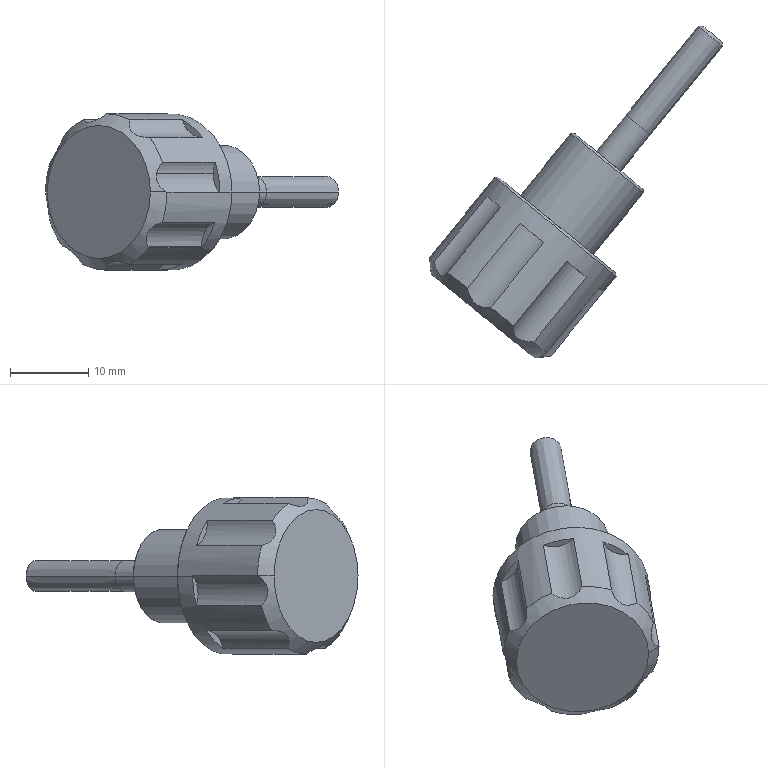Part | SolidWorks | features BaseBody 1 | 1 solid | 38 faces | box 37.447 x 42.447 x 20 mm | volume 5886 mm3 | cylinder 16 | plane 12 | cone 10 | commonest cylinder face diameters 6.478 x10 4 x2 12 x2 20 x2
STEP:
#1=CARTESIAN_POINT('',(523.226,-172.155,255.843));
#2=VERTEX_POINT('',#1);
#3=CARTESIAN_POINT('',(507.709,-159.537,255.843));
#4=VERTEX_POINT('',#3);
#5=CARTESIAN_POINT('',(515.467,-165.846,255.843));
#6=DIRECTION('',(-0.6309,-0.7758,0.000000012));
#7=DIRECTION('',(0.7758,-0.6309,0.));
#8=AXIS2_PLACEMENT_3D('',#5,#6,#7);
#9=CIRCLE('',#8,10.);
#10=EDGE_CURVE('',#2,#4,#9,.T.);
#11=ORIENTED_EDGE('',*,*,#10,.T.);
#12=CARTESIAN_POINT('',(506.127,-161.482,255.843));
#13=VERTEX_POINT('',#12);
#14=CARTESIAN_POINT('',(498.434,-170.941,255.843));
#15=DIRECTION('',(-0.6309,-0.7758,0.000000012));
#16=VECTOR('',#15,1000.);
#17=LINE('',#14,#16);
#18=EDGE_CURVE('',#4,#13,#17,.T.);
#19=ORIENTED_EDGE('',*,*,#18,.T.);
#20=CARTESIAN_POINT('',(506.127,-161.482,255.944));
#21=VERTEX_POINT('',#20);
#22=CARTESIAN_POINT('',(513.885,-167.791,255.843));
#23=DIRECTION('',(0.6309,0.7758,-0.000000012));
#24=DIRECTION('',(0.7758,-0.6309,0.));
#25=AXIS2_PLACEMENT_3D('',#22,#23,#24);
#26=CIRCLE('',#25,10.);
#27=EDGE_CURVE('',#13,#21,#26,.T.);
#28=ORIENTED_EDGE('',*,*,#27,.T.);
#29=CARTESIAN_POINT('',(499.381,-169.778,255.944));
#30=VERTEX_POINT('',#29);
#31=CARTESIAN_POINT('',(498.434,-170.942,255.944));
#32=DIRECTION('',(-0.6309,-0.7758,0.000000012));
#33=VECTOR('',#32,1000.);
#34=LINE('',#31,#33);
#35=EDGE_CURVE('',#21,#30,#34,.T.);
#36=ORIENTED_EDGE('',*,*,#35,.T.);
#37=CARTESIAN_POINT('',(499.988,-170.272,259.722));
#38=VERTEX_POINT('',#37);
#39=CARTESIAN_POINT('',(507.139,-176.087,255.843));
#40=DIRECTION('',(0.6309,0.7758,-0.000000012));
#41=DIRECTION('',(0.7758,-0.6309,0.));
#42=AXIS2_PLACEMENT_3D('',#39,#40,#41);
#43=CIRCLE('',#42,10.);
#44=EDGE_CURVE('',#30,#38,#43,.T.);
#45=ORIENTED_EDGE('',*,*,#44,.T.);
#46=CARTESIAN_POINT('',(506.734,-161.976,259.722));
#47=VERTEX_POINT('',#46);
#48=CARTESIAN_POINT('',(499.041,-171.435,259.722));
#49=DIRECTION('',(0.6309,0.7758,-0.000000012));
#50=VECTOR('',#49,1000.);
#51=LINE('',#48,#50);
#52=EDGE_CURVE('',#38,#47,#51,.T.);
#53=ORIENTED_EDGE('',*,*,#52,.T.);
#54=CARTESIAN_POINT('',(508.454,-163.375,262.985));
#55=VERTEX_POINT('',#54);
#56=CARTESIAN_POINT('',(513.885,-167.791,255.843));
#57=DIRECTION('',(0.6309,0.7758,-0.000000012));
#58=DIRECTION('',(0.7758,-0.6309,0.));
#59=AXIS2_PLACEMENT_3D('',#56,#57,#58);
#60=CIRCLE('',#59,10.);
#61=EDGE_CURVE('',#47,#55,#60,.T.);
#62=ORIENTED_EDGE('',*,*,#61,.T.);
#63=CARTESIAN_POINT('',(501.708,-171.671,262.985));
#64=VERTEX_POINT('',#63);
#65=CARTESIAN_POINT('',(500.762,-172.834,262.985));
#66=DIRECTION('',(-0.6309,-0.7758,0.000000012));
#67=VECTOR('',#66,1000.);
#68=LINE('',#65,#67);
#69=EDGE_CURVE('',#55,#64,#68,.T.);
#70=ORIENTED_EDGE('',*,*,#69,.T.);
#71=CARTESIAN_POINT('',(504.21,-173.705,265.104));
#72=VERTEX_POINT('',#71);
#73=CARTESIAN_POINT('',(507.139,-176.087,255.843));
#74=DIRECTION('',(0.6309,0.7758,-0.000000012));
#75=DIRECTION('',(0.7758,-0.6309,0.));
#76=AXIS2_PLACEMENT_3D('',#73,#74,#75);
#77=CIRCLE('',#76,10.);
#78=EDGE_CURVE('',#64,#72,#77,.T.);
#79=ORIENTED_EDGE('',*,*,#78,.T.);
#80=CARTESIAN_POINT('',(510.956,-165.41,265.104));
#81=VERTEX_POINT('',#80);
#82=CARTESIAN_POINT('',(503.264,-174.869,265.104));
#83=DIRECTION('',(0.6309,0.7758,-0.000000012));
#84=VECTOR('',#83,1000.);
#85=LINE('',#82,#84);
#86=EDGE_CURVE('',#72,#81,#85,.T.);
#87=ORIENTED_EDGE('',*,*,#86,.T.);
#88=CARTESIAN_POINT('',(513.963,-167.855,265.843));
#89=VERTEX_POINT('',#88);
#90=CARTESIAN_POINT('',(513.885,-167.791,255.843));
#91=DIRECTION('',(0.6309,0.7758,-0.000000012));
#92=DIRECTION('',(0.7758,-0.6309,0.));
#93=AXIS2_PLACEMENT_3D('',#90,#91,#92);
#94=CIRCLE('',#93,10.);
#95=EDGE_CURVE('',#81,#89,#94,.T.);
#96=ORIENTED_EDGE('',*,*,#95,.T.);
#97=CARTESIAN_POINT('',(507.217,-176.15,265.843));
#98=VERTEX_POINT('',#97);
#99=CARTESIAN_POINT('',(506.271,-177.314,265.843));
#100=DIRECTION('',(-0.6309,-0.7758,0.000000012));
#101=VECTOR('',#100,1000.);
#102=LINE('',#99,#101);
#103=EDGE_CURVE('',#89,#98,#102,.T.);
#104=ORIENTED_EDGE('',*,*,#103,.T.);
#105=CARTESIAN_POINT('',(510.148,-178.534,265.06));
#106=VERTEX_POINT('',#105);
#107=CARTESIAN_POINT('',(507.139,-176.087,255.843));
#108=DIRECTION('',(0.6309,0.7758,-0.000000012));
#109=DIRECTION('',(0.7758,-0.6309,0.));
#110=AXIS2_PLACEMENT_3D('',#107,#108,#109);
#111=CIRCLE('',#110,10.);
#112=EDGE_CURVE('',#98,#106,#111,.T.);
#113=ORIENTED_EDGE('',*,*,#112,.T.);
#114=CARTESIAN_POINT('',(516.894,-170.239,265.06));
#115=VERTEX_POINT('',#114);
#116=CARTESIAN_POINT('',(509.202,-179.698,265.06));
#117=DIRECTION('',(0.6309,0.7758,-0.000000012));
#118=VECTOR('',#117,1000.);
#119=LINE('',#116,#118);
#120=EDGE_CURVE('',#106,#115,#119,.T.);
#121=ORIENTED_EDGE('',*,*,#120,.T.);
#122=CARTESIAN_POINT('',(519.426,-172.297,262.843));
#123=VERTEX_POINT('',#122);
#124=CARTESIAN_POINT('',(513.885,-167.791,255.843));
#125=DIRECTION('',(0.6309,0.7758,-0.000000012));
#126=DIRECTION('',(0.7758,-0.6309,0.));
#127=AXIS2_PLACEMENT_3D('',#124,#125,#126);
#128=CIRCLE('',#127,10.);
#129=EDGE_CURVE('',#115,#123,#128,.T.);
#130=ORIENTED_EDGE('',*,*,#129,.T.);
#131=CARTESIAN_POINT('',(512.68,-180.593,262.843));
#132=VERTEX_POINT('',#131);
#133=CARTESIAN_POINT('',(511.733,-181.757,262.843));
#134=DIRECTION('',(-0.6309,-0.7758,0.000000012));
#135=VECTOR('',#134,1000.);
#136=LINE('',#133,#135);
#137=EDGE_CURVE('',#123,#132,#136,.T.);
#138=ORIENTED_EDGE('',*,*,#137,.T.);
#139=CARTESIAN_POINT('',(514.323,-181.929,259.618));
#140=VERTEX_POINT('',#139);
#141=CARTESIAN_POINT('',(507.139,-176.087,255.843));
#142=DIRECTION('',(0.6309,0.7758,-0.000000012));
#143=DIRECTION('',(0.7758,-0.6309,0.));
#144=AXIS2_PLACEMENT_3D('',#141,#142,#143);
#145=CIRCLE('',#144,10.);
#146=EDGE_CURVE('',#132,#140,#145,.T.);
#147=ORIENTED_EDGE('',*,*,#146,.T.);
#148=CARTESIAN_POINT('',(521.069,-173.634,259.618));
#149=VERTEX_POINT('',#148);
#150=CARTESIAN_POINT('',(513.377,-183.093,259.618));
#151=DIRECTION('',(0.6309,0.7758,-0.000000012));
#152=VECTOR('',#151,1000.);
#153=LINE('',#150,#152);
#154=EDGE_CURVE('',#140,#149,#153,.T.);
#155=ORIENTED_EDGE('',*,*,#154,.T.);
#156=CARTESIAN_POINT('',(521.643,-174.101,255.843));
#157=VERTEX_POINT('',#156);
#158=CARTESIAN_POINT('',(513.885,-167.791,255.843));
#159=DIRECTION('',(0.6309,0.7758,-0.000000012));
#160=DIRECTION('',(0.7758,-0.6309,0.));
#161=AXIS2_PLACEMENT_3D('',#158,#159,#160);
#162=CIRCLE('',#161,10.);
#163=EDGE_CURVE('',#149,#157,#162,.T.);
#164=ORIENTED_EDGE('',*,*,#163,.T.);
#165=CARTESIAN_POINT('',(513.951,-183.56,255.843));
#166=DIRECTION('',(-0.6309,-0.7758,0.000000012));
#167=VECTOR('',#166,1000.);
#168=LINE('',#165,#167);
#169=EDGE_CURVE('',#2,#157,#168,.T.);
#170=ORIENTED_EDGE('',*,*,#169,.F.);
#171=EDGE_LOOP('',(#11,#19,#28,#36,#45,#53,#62,#70,#79,#87,#96,#104,#113,#121,#130,#138,#147,#155,#164,#170));
#172=FACE_OUTER_BOUND('',#171,.T.);
#173=CARTESIAN_POINT('',(506.192,-177.251,255.843));
#174=DIRECTION('',(-0.6309,-0.7758,0.000000012));
#175=DIRECTION('',(0.7758,-0.6309,0.));
#176=AXIS2_PLACEMENT_3D('',#173,#174,#175);
#177=CYLINDRICAL_SURFACE('',#176,10.);
#178=ADVANCED_FACE('',(#172),#177,.T.);
#179=CARTESIAN_POINT('',(499.598,-171.888,255.843));
#180=VERTEX_POINT('',#179);
#181=CARTESIAN_POINT('',(512.787,-182.614,255.843));
#182=VERTEX_POINT('',#181);
#183=CARTESIAN_POINT('',(506.192,-177.251,255.843));
#184=DIRECTION('',(0.6309,0.7758,-0.000000012));
#185=DIRECTION('',(-0.7758,0.6309,0.));
#186=AXIS2_PLACEMENT_3D('',#183,#184,#185);
#187=CIRCLE('',#186,8.5);
#188=EDGE_CURVE('',#180,#182,#187,.T.);
#189=ORIENTED_EDGE('',*,*,#188,.T.);
#190=CARTESIAN_POINT('',(514.745,-182.412,255.843));
#191=VERTEX_POINT('',#190);
#192=CARTESIAN_POINT('',(514.897,-182.396,255.843));
#193=DIRECTION('',(0.9947,0.1025,-0.000000009));
#194=VECTOR('',#193,1000.);
#195=LINE('',#192,#194);
#196=EDGE_CURVE('',#182,#191,#195,.T.);
#197=ORIENTED_EDGE('',*,*,#196,.T.);
#198=CARTESIAN_POINT('',(513.557,-182.323,258.162));
#199=VERTEX_POINT('',#198);
#200=CARTESIAN_POINT('',(514.745,-182.412,255.843));
#201=CARTESIAN_POINT('',(514.556,-182.431,255.974));
#202=CARTESIAN_POINT('',(514.379,-182.448,256.12));
#203=CARTESIAN_POINT('',(514.058,-182.47,256.452));
#204=CARTESIAN_POINT('',(513.915,-182.475,256.636));
#205=CARTESIAN_POINT('',(513.746,-182.469,256.937));
#206=CARTESIAN_POINT('',(513.697,-182.464,257.043));
#207=CARTESIAN_POINT('',(513.617,-182.45,257.259));
#208=CARTESIAN_POINT('',(513.586,-182.441,257.369));
#209=CARTESIAN_POINT('',(513.523,-182.404,257.704));
#210=CARTESIAN_POINT('',(513.522,-182.367,257.938));
#211=CARTESIAN_POINT('',(513.557,-182.323,258.162));
#212=B_SPLINE_CURVE_WITH_KNOTS('',3,(#200,#201,#202,#203,#204,#205,#206,#207,#208,#209,#210,#211),.UNSPECIFIED.,.F.,.F.,(4,2,2,2,2,4),(0.0001822,0.0008713,0.00156,0.001905,0.00225,0.002939),.UNSPECIFIED.);
#213=EDGE_CURVE('',#191,#199,#212,.T.);
#214=ORIENTED_EDGE('',*,*,#213,.T.);
#215=CARTESIAN_POINT('',(513.557,-182.323,258.162));
#216=CARTESIAN_POINT('',(513.579,-182.296,258.3));
#217=CARTESIAN_POINT('',(513.615,-182.266,258.437));
#218=CARTESIAN_POINT('',(513.709,-182.203,258.7));
#219=CARTESIAN_POINT('',(513.767,-182.17,258.825));
#220=CARTESIAN_POINT('',(513.966,-182.069,259.188));
#221=CARTESIAN_POINT('',(514.134,-181.999,259.413));
#222=CARTESIAN_POINT('',(514.323,-181.929,259.618));
#223=B_SPLINE_CURVE_WITH_KNOTS('',3,(#215,#216,#217,#218,#219,#220,#221,#222),.UNSPECIFIED.,.F.,.F.,(4,2,2,4),(0.002939,0.003365,0.003792,0.004644),.UNSPECIFIED.);
#224=EDGE_CURVE('',#199,#140,#223,.T.);
#225=ORIENTED_EDGE('',*,*,#224,.T.);
#226=ORIENTED_EDGE('',*,*,#146,.F.);
#227=CARTESIAN_POINT('',(512.68,-180.593,262.843));
#228=CARTESIAN_POINT('',(512.485,-180.586,262.834));
#229=CARTESIAN_POINT('',(512.292,-180.571,262.836));
#230=CARTESIAN_POINT('',(511.909,-180.523,262.865));
#231=CARTESIAN_POINT('',(511.717,-180.489,262.893));
#232=CARTESIAN_POINT('',(511.35,-180.396,262.981));
#233=CARTESIAN_POINT('',(511.175,-180.337,263.039));
#234=CARTESIAN_POINT('',(510.847,-180.189,263.194));
#235=CARTESIAN_POINT('',(510.7,-180.1,263.288));
#236=CARTESIAN_POINT('',(510.448,-179.895,263.509));
#237=CARTESIAN_POINT('',(510.349,-179.783,263.63));
#238=CARTESIAN_POINT('',(510.197,-179.544,263.893));
#239=CARTESIAN_POINT('',(510.145,-179.417,264.035));
#240=CARTESIAN_POINT('',(510.085,-179.163,264.322));
#241=CARTESIAN_POINT('',(510.075,-179.034,264.469));
#242=CARTESIAN_POINT('',(510.089,-178.781,264.764));
#243=CARTESIAN_POINT('',(510.112,-178.656,264.912));
#244=CARTESIAN_POINT('',(510.148,-178.534,265.06));
#245=B_SPLINE_CURVE_WITH_KNOTS('',3,(#227,#228,#229,#230,#231,#232,#233,#234,#235,#236,#237,#238,#239,#240,#241,#242,#243,#244),.UNSPECIFIED.,.F.,.F.,(4,2,2,2,2,2,2,2,4),(0.,0.0005805,0.001161,0.001742,0.002322,0.002903,0.003483,0.004064,0.004644),.UNSPECIFIED.);
#246=EDGE_CURVE('',#132,#106,#245,.T.);
#247=ORIENTED_EDGE('',*,*,#246,.T.);
#248=ORIENTED_EDGE('',*,*,#112,.F.);
#249=CARTESIAN_POINT('',(507.217,-176.15,265.843));
#250=CARTESIAN_POINT('',(507.062,-176.176,265.726));
#251=CARTESIAN_POINT('',(506.904,-176.19,265.615));
#252=CARTESIAN_POINT('',(506.579,-176.189,265.404));
#253=CARTESIAN_POINT('',(506.411,-176.174,265.304));
#254=CARTESIAN_POINT('',(506.074,-176.106,265.123));
#255=CARTESIAN_POINT('',(505.906,-176.053,265.042));
#256=CARTESIAN_POINT('',(505.573,-175.899,264.905));
#257=CARTESIAN_POINT('',(505.414,-175.801,264.852));
#258=CARTESIAN_POINT('',(505.119,-175.562,264.779));
#259=CARTESIAN_POINT('',(504.982,-175.419,264.76));
#260=CARTESIAN_POINT('',(504.746,-175.111,264.756));
#261=CARTESIAN_POINT('',(504.643,-174.942,264.771));
#262=CARTESIAN_POINT('',(504.387,-174.427,264.855));
#263=CARTESIAN_POINT('',(504.278,-174.064,264.963));
#264=CARTESIAN_POINT('',(504.21,-173.705,265.104));
#265=B_SPLINE_CURVE_WITH_KNOTS('',3,(#249,#250,#251,#252,#253,#254,#255,#256,#257,#258,#259,#260,#261,#262,#263,#264),.UNSPECIFIED.,.F.,.F.,(4,2,2,2,2,2,2,4),(0.,0.0005805,0.001161,0.001742,0.002322,0.002903,0.003483,0.004644),.UNSPECIFIED.);
#266=EDGE_CURVE('',#98,#72,#265,.T.);
#267=ORIENTED_EDGE('',*,*,#266,.T.);
#268=ORIENTED_EDGE('',*,*,#78,.F.);
#269=CARTESIAN_POINT('',(501.708,-171.671,262.985));
#270=CARTESIAN_POINT('',(501.641,-171.768,262.83));
#271=CARTESIAN_POINT('',(501.57,-171.852,262.67));
#272=CARTESIAN_POINT('',(501.418,-171.992,262.343));
#273=CARTESIAN_POINT('',(501.337,-172.048,262.173));
#274=CARTESIAN_POINT('',(501.168,-172.116,261.829));
#275=CARTESIAN_POINT('',(501.082,-172.13,261.656));
#276=CARTESIAN_POINT('',(500.905,-172.103,261.308));
#277=CARTESIAN_POINT('',(500.817,-172.062,261.14));
#278=CARTESIAN_POINT('',(500.648,-171.926,260.82));
#279=CARTESIAN_POINT('',(500.566,-171.828,260.667));
#280=CARTESIAN_POINT('',(500.418,-171.592,260.397));
#281=CARTESIAN_POINT('',(500.35,-171.451,260.276));
#282=CARTESIAN_POINT('',(500.167,-170.995,259.966));
#283=CARTESIAN_POINT('',(500.069,-170.641,259.82));
#284=CARTESIAN_POINT('',(499.988,-170.272,259.722));
#285=B_SPLINE_CURVE_WITH_KNOTS('',3,(#269,#270,#271,#272,#273,#274,#275,#276,#277,#278,#279,#280,#281,#282,#283,#284),.UNSPECIFIED.,.F.,.F.,(4,2,2,2,2,2,2,4),(0.,0.0005805,0.001161,0.001742,0.002322,0.002903,0.003483,0.004644),.UNSPECIFIED.);
#286=EDGE_CURVE('',#64,#38,#285,.T.);
#287=ORIENTED_EDGE('',*,*,#286,.T.);
#288=ORIENTED_EDGE('',*,*,#44,.F.);
#289=CARTESIAN_POINT('',(499.396,-169.93,255.843));
#290=VERTEX_POINT('',#289);
#291=CARTESIAN_POINT('',(499.381,-169.778,255.944));
#292=CARTESIAN_POINT('',(499.386,-169.83,255.911));
#293=CARTESIAN_POINT('',(499.391,-169.88,255.878));
#294=CARTESIAN_POINT('',(499.396,-169.93,255.843));
#295=B_SPLINE_CURVE_WITH_KNOTS('',3,(#291,#292,#293,#294),.UNSPECIFIED.,.F.,.F.,(4,4),(0.,0.0001822),.UNSPECIFIED.);
#296=EDGE_CURVE('',#30,#290,#295,.T.);
#297=ORIENTED_EDGE('',*,*,#296,.T.);
#298=CARTESIAN_POINT('',(499.38,-169.778,255.843));
#299=DIRECTION('',(-0.1025,0.9947,-0.000000009));
#300=VECTOR('',#299,1000.);
#301=LINE('',#298,#300);
#302=EDGE_CURVE('',#180,#290,#301,.T.);
#303=ORIENTED_EDGE('',*,*,#302,.F.);
#304=EDGE_LOOP('',(#189,#197,#214,#225,#226,#247,#248,#267,#268,#287,#288,#297,#303));
#305=FACE_OUTER_BOUND('',#304,.T.);
#306=CARTESIAN_POINT('',(507.139,-176.087,255.843));
#307=DIRECTION('',(0.6309,0.7758,-0.000000012));
#308=DIRECTION('',(-0.7758,0.6309,0.));
#309=AXIS2_PLACEMENT_3D('',#306,#307,#308);
#310=CONICAL_SURFACE('',#309,10.,0.7854);
#311=ADVANCED_FACE('',(#305),#310,.T.);
#312=CARTESIAN_POINT('',(512.479,-180.606,248.889));
#313=VERTEX_POINT('',#312);
#314=CARTESIAN_POINT('',(514.29,-181.902,251.964));
#315=VERTEX_POINT('',#314);
#316=CARTESIAN_POINT('',(512.479,-180.606,248.889));
#317=CARTESIAN_POINT('',(512.412,-180.688,249.04));
#318=CARTESIAN_POINT('',(512.357,-180.772,249.194));
#319=CARTESIAN_POINT('',(512.278,-180.942,249.511));
#320=CARTESIAN_POINT('',(512.254,-181.029,249.676));
#321=CARTESIAN_POINT('',(512.247,-181.196,250.004));
#322=CARTESIAN_POINT('',(512.265,-181.279,250.17));
#323=CARTESIAN_POINT('',(512.349,-181.432,250.496));
#324=CARTESIAN_POINT('',(512.415,-181.502,250.652));
#325=CARTESIAN_POINT('',(512.595,-181.626,250.95));
#326=CARTESIAN_POINT('',(512.709,-181.679,251.09));
#327=CARTESIAN_POINT('',(512.968,-181.766,251.338));
#328=CARTESIAN_POINT('',(513.116,-181.8,251.449));
#329=CARTESIAN_POINT('',(513.582,-181.877,251.735));
#330=CARTESIAN_POINT('',(513.93,-181.898,251.871));
#331=CARTESIAN_POINT('',(514.29,-181.902,251.964));
#332=B_SPLINE_CURVE_WITH_KNOTS('',3,(#316,#317,#318,#319,#320,#321,#322,#323,#324,#325,#326,#327,#328,#329,#330,#331),.UNSPECIFIED.,.F.,.F.,(4,2,2,2,2,2,2,4),(0.0002308,0.0007825,0.001334,0.001886,0.002438,0.002989,0.003541,0.004644),.UNSPECIFIED.);
#333=EDGE_CURVE('',#313,#315,#332,.T.);
#334=ORIENTED_EDGE('',*,*,#333,.F.);
#335=CARTESIAN_POINT('',(519.311,-172.204,248.889));
#336=VERTEX_POINT('',#335);
#337=CARTESIAN_POINT('',(511.619,-181.663,248.889));
#338=DIRECTION('',(0.6309,0.7758,-0.000000012));
#339=VECTOR('',#338,1000.);
#340=LINE('',#337,#339);
#341=EDGE_CURVE('',#313,#336,#340,.T.);
#342=ORIENTED_EDGE('',*,*,#341,.T.);
#343=CARTESIAN_POINT('',(521.036,-173.607,251.964));
#344=VERTEX_POINT('',#343);
#345=CARTESIAN_POINT('',(521.824,-174.248,248.889));
#346=DIRECTION('',(-0.6309,-0.7758,0.000000012));
#347=DIRECTION('',(-0.7758,0.6309,0.));
#348=AXIS2_PLACEMENT_3D('',#345,#346,#347);
#349=CIRCLE('',#348,3.239);
#350=EDGE_CURVE('',#344,#336,#349,.T.);
#351=ORIENTED_EDGE('',*,*,#350,.F.);
#352=CARTESIAN_POINT('',(513.343,-183.066,251.964));
#353=DIRECTION('',(0.6309,0.7758,-0.000000012));
#354=VECTOR('',#353,1000.);
#355=LINE('',#352,#354);
#356=EDGE_CURVE('',#315,#344,#355,.T.);
#357=ORIENTED_EDGE('',*,*,#356,.F.);
#358=EDGE_LOOP('',(#334,#342,#351,#357));
#359=FACE_OUTER_BOUND('',#358,.T.);
#360=CARTESIAN_POINT('',(514.132,-183.707,248.889));
#361=DIRECTION('',(0.6309,0.7758,-0.000000012));
#362=DIRECTION('',(-0.7758,0.6309,0.));
#363=AXIS2_PLACEMENT_3D('',#360,#361,#362);
#364=CYLINDRICAL_SURFACE('',#363,3.239);
#365=ADVANCED_FACE('',(#359),#364,.F.);
#366=ORIENTED_EDGE('',*,*,#224,.F.);
#367=CARTESIAN_POINT('',(520.801,-173.416,258.162));
#368=VERTEX_POINT('',#367);
#369=CARTESIAN_POINT('',(513.109,-182.875,258.162));
#370=DIRECTION('',(0.6309,0.7758,-0.000000012));
#371=VECTOR('',#370,1000.);
#372=LINE('',#369,#371);
#373=EDGE_CURVE('',#199,#368,#372,.T.);
#374=ORIENTED_EDGE('',*,*,#373,.T.);
#375=CARTESIAN_POINT('',(523.314,-175.459,258.162));
#376=DIRECTION('',(-0.6309,-0.7758,0.000000012));
#377=DIRECTION('',(-0.7758,0.6309,0.));
#378=AXIS2_PLACEMENT_3D('',#375,#376,#377);
#379=CIRCLE('',#378,3.239);
#380=EDGE_CURVE('',#149,#368,#379,.T.);
#381=ORIENTED_EDGE('',*,*,#380,.F.);
#382=ORIENTED_EDGE('',*,*,#154,.F.);
#383=EDGE_LOOP('',(#366,#374,#381,#382));
#384=FACE_OUTER_BOUND('',#383,.T.);
#385=CARTESIAN_POINT('',(515.622,-184.919,258.162));
#386=DIRECTION('',(0.6309,0.7758,-0.000000012));
#387=DIRECTION('',(-0.7758,0.6309,0.));
#388=AXIS2_PLACEMENT_3D('',#385,#386,#387);
#389=CYLINDRICAL_SURFACE('',#388,3.239);
#390=ADVANCED_FACE('',(#384),#389,.F.);
#391=CARTESIAN_POINT('',(523.182,-171.733,255.843));
#392=VERTEX_POINT('',#391);
#393=CARTESIAN_POINT('',(508.131,-159.493,255.843));
#394=VERTEX_POINT('',#393);
#395=CARTESIAN_POINT('',(515.656,-165.613,255.843));
#396=DIRECTION('',(-0.6309,-0.7758,0.000000012));
#397=DIRECTION('',(0.7758,-0.6309,0.));
#398=AXIS2_PLACEMENT_3D('',#395,#396,#397);
#399=CIRCLE('',#398,9.7);
#400=EDGE_CURVE('',#392,#394,#399,.T.);
#401=ORIENTED_EDGE('',*,*,#400,.T.);
#402=CARTESIAN_POINT('',(507.709,-159.537,255.843));
#403=DIRECTION('',(-0.9947,-0.1025,0.000000009));
#404=VECTOR('',#403,1000.);
#405=LINE('',#402,#404);
#406=EDGE_CURVE('',#394,#4,#405,.T.);
#407=ORIENTED_EDGE('',*,*,#406,.T.);
#408=ORIENTED_EDGE('',*,*,#10,.F.);
#409=CARTESIAN_POINT('',(523.226,-172.155,255.843));
#410=DIRECTION('',(0.1025,-0.9947,0.000000009));
#411=VECTOR('',#410,1000.);
#412=LINE('',#409,#411);
#413=EDGE_CURVE('',#392,#2,#412,.T.);
#414=ORIENTED_EDGE('',*,*,#413,.F.);
#415=EDGE_LOOP('',(#401,#407,#408,#414));
#416=FACE_OUTER_BOUND('',#415,.T.);
#417=CARTESIAN_POINT('',(515.467,-165.846,255.843));
#418=DIRECTION('',(-0.6309,-0.7758,0.000000012));
#419=DIRECTION('',(0.7758,-0.6309,0.));
#420=AXIS2_PLACEMENT_3D('',#417,#418,#419);
#421=CONICAL_SURFACE('',#420,10.,0.7854);
#422=ADVANCED_FACE('',(#416),#421,.T.);
#423=CARTESIAN_POINT('',(526.747,-161.485,255.843));
#424=VERTEX_POINT('',#423);
#425=CARTESIAN_POINT('',(517.437,-153.914,255.843));
#426=VERTEX_POINT('',#425);
#427=CARTESIAN_POINT('',(522.092,-157.7,255.843));
#428=DIRECTION('',(-0.6309,-0.7758,0.000000012));
#429=DIRECTION('',(0.7758,-0.6309,0.));
#430=AXIS2_PLACEMENT_3D('',#427,#428,#429);
#431=CIRCLE('',#430,6.);
#432=EDGE_CURVE('',#424,#426,#431,.T.);
#433=ORIENTED_EDGE('',*,*,#432,.T.);
#434=CARTESIAN_POINT('',(511.001,-161.828,255.843));
#435=VERTEX_POINT('',#434);
#436=CARTESIAN_POINT('',(511.001,-161.828,255.843));
#437=DIRECTION('',(-0.6309,-0.7758,0.000000012));
#438=VECTOR('',#437,1000.);
#439=LINE('',#436,#438);
#440=EDGE_CURVE('',#426,#435,#439,.T.);
#441=ORIENTED_EDGE('',*,*,#440,.T.);
#442=CARTESIAN_POINT('',(520.311,-169.399,255.843));
#443=VERTEX_POINT('',#442);
#444=CARTESIAN_POINT('',(515.656,-165.613,255.843));
#445=DIRECTION('',(-0.6309,-0.7758,0.000000012));
#446=DIRECTION('',(0.7758,-0.6309,0.));
#447=AXIS2_PLACEMENT_3D('',#444,#445,#446);
#448=CIRCLE('',#447,6.);
#449=EDGE_CURVE('',#443,#435,#448,.T.);
#450=ORIENTED_EDGE('',*,*,#449,.F.);
#451=CARTESIAN_POINT('',(520.311,-169.399,255.843));
#452=DIRECTION('',(-0.6309,-0.7758,0.000000012));
#453=VECTOR('',#452,1000.);
#454=LINE('',#451,#453);
#455=EDGE_CURVE('',#424,#443,#454,.T.);
#456=ORIENTED_EDGE('',*,*,#455,.F.);
#457=EDGE_LOOP('',(#433,#441,#450,#456));
#458=FACE_OUTER_BOUND('',#457,.T.);
#459=CARTESIAN_POINT('',(515.656,-165.613,255.843));
#460=DIRECTION('',(-0.6309,-0.7758,0.000000012));
#461=DIRECTION('',(0.7758,-0.6309,0.));
#462=AXIS2_PLACEMENT_3D('',#459,#460,#461);
#463=CYLINDRICAL_SURFACE('',#462,6.);
#464=ADVANCED_FACE('',(#458),#463,.T.);
#465=CARTESIAN_POINT('',(526.703,-161.063,255.843));
#466=VERTEX_POINT('',#465);
#467=CARTESIAN_POINT('',(517.859,-153.87,255.843));
#468=VERTEX_POINT('',#467);
#469=CARTESIAN_POINT('',(522.281,-157.467,255.843));
#470=DIRECTION('',(-0.6309,-0.7758,0.000000012));
#471=DIRECTION('',(0.7758,-0.6309,0.));
#472=AXIS2_PLACEMENT_3D('',#469,#470,#471);
#473=CIRCLE('',#472,5.7);
#474=EDGE_CURVE('',#466,#468,#473,.T.);
#475=ORIENTED_EDGE('',*,*,#474,.T.);
#476=CARTESIAN_POINT('',(517.437,-153.914,255.843));
#477=DIRECTION('',(-0.9947,-0.1025,0.000000009));
#478=VECTOR('',#477,1000.);
#479=LINE('',#476,#478);
#480=EDGE_CURVE('',#468,#426,#479,.T.);
#481=ORIENTED_EDGE('',*,*,#480,.T.);
#482=ORIENTED_EDGE('',*,*,#432,.F.);
#483=CARTESIAN_POINT('',(526.747,-161.485,255.843));
#484=DIRECTION('',(0.1025,-0.9947,0.000000009));
#485=VECTOR('',#484,1000.);
#486=LINE('',#483,#485);
#487=EDGE_CURVE('',#466,#424,#486,.T.);
#488=ORIENTED_EDGE('',*,*,#487,.F.);
#489=EDGE_LOOP('',(#475,#481,#482,#488));
#490=FACE_OUTER_BOUND('',#489,.T.);
#491=CARTESIAN_POINT('',(522.092,-157.7,255.843));
#492=DIRECTION('',(-0.6309,-0.7758,0.000000012));
#493=DIRECTION('',(0.7758,-0.6309,0.));
#494=AXIS2_PLACEMENT_3D('',#491,#492,#493);
#495=CONICAL_SURFACE('',#494,6.,0.7854);
#496=ADVANCED_FACE('',(#490),#495,.T.);
#497=CARTESIAN_POINT('',(527.618,-154.074,255.843));
#498=VERTEX_POINT('',#497);
#499=CARTESIAN_POINT('',(524.515,-151.55,255.843));
#500=VERTEX_POINT('',#499);
#501=CARTESIAN_POINT('',(526.067,-152.812,255.843));
#502=DIRECTION('',(-0.6309,-0.7758,0.000000012));
#503=DIRECTION('',(0.7758,-0.6309,0.));
#504=AXIS2_PLACEMENT_3D('',#501,#502,#503);
#505=CIRCLE('',#504,2.);
#506=EDGE_CURVE('',#498,#500,#505,.T.);
#507=ORIENTED_EDGE('',*,*,#506,.T.);
#508=CARTESIAN_POINT('',(520.729,-156.205,255.843));
#509=VERTEX_POINT('',#508);
#510=CARTESIAN_POINT('',(520.729,-156.205,255.843));
#511=DIRECTION('',(-0.6309,-0.7758,0.000000012));
#512=VECTOR('',#511,1000.);
#513=LINE('',#510,#512);
#514=EDGE_CURVE('',#500,#509,#513,.T.);
#515=ORIENTED_EDGE('',*,*,#514,.T.);
#516=CARTESIAN_POINT('',(523.833,-158.729,255.843));
#517=VERTEX_POINT('',#516);
#518=CARTESIAN_POINT('',(522.281,-157.467,255.843));
#519=DIRECTION('',(-0.6309,-0.7758,0.000000012));
#520=DIRECTION('',(0.7758,-0.6309,0.));
#521=AXIS2_PLACEMENT_3D('',#518,#519,#520);
#522=CIRCLE('',#521,2.);
#523=EDGE_CURVE('',#517,#509,#522,.T.);
#524=ORIENTED_EDGE('',*,*,#523,.F.);
#525=CARTESIAN_POINT('',(523.833,-158.729,255.843));
#526=DIRECTION('',(-0.6309,-0.7758,0.000000012));
#527=VECTOR('',#526,1000.);
#528=LINE('',#525,#527);
#529=EDGE_CURVE('',#498,#517,#528,.T.);
#530=ORIENTED_EDGE('',*,*,#529,.F.);
#531=EDGE_LOOP('',(#507,#515,#524,#530));
#532=FACE_OUTER_BOUND('',#531,.T.);
#533=CARTESIAN_POINT('',(522.281,-157.467,255.843));
#534=DIRECTION('',(-0.6309,-0.7758,0.000000012));
#535=DIRECTION('',(0.7758,-0.6309,0.));
#536=AXIS2_PLACEMENT_3D('',#533,#534,#535);
#537=CYLINDRICAL_SURFACE('',#536,2.);
#538=ADVANCED_FACE('',(#532),#537,.T.);
#539=CARTESIAN_POINT('',(536.828,-142.745,255.843));
#540=VERTEX_POINT('',#539);
#541=CARTESIAN_POINT('',(533.729,-140.224,255.843));
#542=VERTEX_POINT('',#541);
#543=CARTESIAN_POINT('',(535.278,-141.484,255.843));
#544=DIRECTION('',(-0.6309,-0.7758,0.000000012));
#545=DIRECTION('',(-0.4361,0.3546,-0.8271));
#546=AXIS2_PLACEMENT_3D('',#543,#544,#545);
#547=CIRCLE('',#546,1.997);
#548=EDGE_CURVE('',#540,#542,#547,.T.);
#549=ORIENTED_EDGE('',*,*,#548,.T.);
#550=CARTESIAN_POINT('',(524.515,-151.55,255.843));
#551=DIRECTION('',(-0.6311,-0.7757,0.000000012));
#552=VECTOR('',#551,1000.);
#553=LINE('',#550,#552);
#554=EDGE_CURVE('',#542,#500,#553,.T.);
#555=ORIENTED_EDGE('',*,*,#554,.T.);
#556=ORIENTED_EDGE('',*,*,#506,.F.);
#557=CARTESIAN_POINT('',(527.618,-154.074,255.843));
#558=DIRECTION('',(-0.6308,-0.7759,0.000000012));
#559=VECTOR('',#558,1000.);
#560=LINE('',#557,#559);
#561=EDGE_CURVE('',#540,#498,#560,.T.);
#562=ORIENTED_EDGE('',*,*,#561,.F.);
#563=EDGE_LOOP('',(#549,#555,#556,#562));
#564=FACE_OUTER_BOUND('',#563,.T.);
#565=CARTESIAN_POINT('',(526.067,-152.812,255.843));
#566=DIRECTION('',(-0.6309,-0.7758,0.000000012));
#567=DIRECTION('',(0.7758,-0.6309,0.));
#568=AXIS2_PLACEMENT_3D('',#565,#566,#567);
#569=CONICAL_SURFACE('',#568,2.,0.0001745);
#570=ADVANCED_FACE('',(#564),#569,.T.);
#571=CARTESIAN_POINT('',(536.77,-142.182,255.843));
#572=VERTEX_POINT('',#571);
#573=CARTESIAN_POINT('',(534.291,-140.166,255.843));
#574=VERTEX_POINT('',#573);
#575=CARTESIAN_POINT('',(535.531,-141.174,255.843));
#576=DIRECTION('',(-0.6309,-0.7758,0.000000012));
#577=DIRECTION('',(0.7758,-0.6309,0.));
#578=AXIS2_PLACEMENT_3D('',#575,#576,#577);
#579=CIRCLE('',#578,1.597);
#580=EDGE_CURVE('',#572,#574,#579,.T.);
#581=ORIENTED_EDGE('',*,*,#580,.T.);
#582=CARTESIAN_POINT('',(533.729,-140.224,255.843));
#583=DIRECTION('',(-0.9947,-0.1024,0.000000009));
#584=VECTOR('',#583,1000.);
#585=LINE('',#582,#584);
#586=EDGE_CURVE('',#574,#542,#585,.T.);
#587=ORIENTED_EDGE('',*,*,#586,.T.);
#588=ORIENTED_EDGE('',*,*,#548,.F.);
#589=CARTESIAN_POINT('',(536.828,-142.745,255.843));
#590=DIRECTION('',(0.1026,-0.9947,0.000000009));
#591=VECTOR('',#590,1000.);
#592=LINE('',#589,#591);
#593=EDGE_CURVE('',#572,#540,#592,.T.);
#594=ORIENTED_EDGE('',*,*,#593,.F.);
#595=EDGE_LOOP('',(#581,#587,#588,#594));
#596=FACE_OUTER_BOUND('',#595,.T.);
#597=CARTESIAN_POINT('',(535.278,-141.484,255.843));
#598=DIRECTION('',(-0.6309,-0.7758,0.000000012));
#599=DIRECTION('',(0.7758,-0.6309,0.));
#600=AXIS2_PLACEMENT_3D('',#597,#598,#599);
#601=CONICAL_SURFACE('',#600,1.997,0.7855);
#602=ADVANCED_FACE('',(#596),#601,.T.);
#603=ORIENTED_EDGE('',*,*,#18,.F.);
#604=CARTESIAN_POINT('',(515.467,-165.846,255.843));
#605=DIRECTION('',(-0.6309,-0.7758,0.000000012));
#606=DIRECTION('',(0.7758,-0.6309,0.));
#607=AXIS2_PLACEMENT_3D('',#604,#605,#606);
#608=CIRCLE('',#607,10.);
#609=EDGE_CURVE('',#4,#2,#608,.T.);
#610=ORIENTED_EDGE('',*,*,#609,.T.);
#611=ORIENTED_EDGE('',*,*,#169,.T.);
#612=CARTESIAN_POINT('',(521.643,-174.1,255.743));
#613=VERTEX_POINT('',#612);
#614=CARTESIAN_POINT('',(513.885,-167.791,255.843));
#615=DIRECTION('',(0.6309,0.7758,-0.000000012));
#616=DIRECTION('',(0.7758,-0.6309,0.));
#617=AXIS2_PLACEMENT_3D('',#614,#615,#616);
#618=CIRCLE('',#617,10.);
#619=EDGE_CURVE('',#157,#613,#618,.T.);
#620=ORIENTED_EDGE('',*,*,#619,.T.);
#621=CARTESIAN_POINT('',(514.897,-182.396,255.743));
#622=VERTEX_POINT('',#621);
#623=CARTESIAN_POINT('',(513.95,-183.56,255.743));
#624=DIRECTION('',(-0.6309,-0.7758,0.000000012));
#625=VECTOR('',#624,1000.);
#626=LINE('',#623,#625);
#627=EDGE_CURVE('',#613,#622,#626,.T.);
#628=ORIENTED_EDGE('',*,*,#627,.T.);
#629=CARTESIAN_POINT('',(507.139,-176.087,255.843));
#630=DIRECTION('',(0.6309,0.7758,-0.000000012));
#631=DIRECTION('',(0.7758,-0.6309,0.));
#632=AXIS2_PLACEMENT_3D('',#629,#630,#631);
#633=CIRCLE('',#632,10.);
#634=EDGE_CURVE('',#622,#315,#633,.T.);
#635=ORIENTED_EDGE('',*,*,#634,.T.);
#636=ORIENTED_EDGE('',*,*,#356,.T.);
#637=CARTESIAN_POINT('',(519.315,-172.208,248.701));
#638=VERTEX_POINT('',#637);
#639=CARTESIAN_POINT('',(513.885,-167.791,255.843));
#640=DIRECTION('',(0.6309,0.7758,-0.000000012));
#641=DIRECTION('',(0.7758,-0.6309,0.));
#642=AXIS2_PLACEMENT_3D('',#639,#640,#641);
#643=CIRCLE('',#642,10.);
#644=EDGE_CURVE('',#344,#638,#643,.T.);
#645=ORIENTED_EDGE('',*,*,#644,.T.);
#646=CARTESIAN_POINT('',(512.569,-180.503,248.701));
#647=VERTEX_POINT('',#646);
#648=CARTESIAN_POINT('',(511.623,-181.667,248.701));
#649=DIRECTION('',(-0.6309,-0.7758,0.000000012));
#650=VECTOR('',#649,1000.);
#651=LINE('',#648,#650);
#652=EDGE_CURVE('',#638,#647,#651,.T.);
#653=ORIENTED_EDGE('',*,*,#652,.T.);
#654=CARTESIAN_POINT('',(510.067,-178.468,246.583));
#655=VERTEX_POINT('',#654);
#656=CARTESIAN_POINT('',(507.139,-176.087,255.843));
#657=DIRECTION('',(0.6309,0.7758,-0.000000012));
#658=DIRECTION('',(0.7758,-0.6309,0.));
#659=AXIS2_PLACEMENT_3D('',#656,#657,#658);
#660=CIRCLE('',#659,10.);
#661=EDGE_CURVE('',#647,#655,#660,.T.);
#662=ORIENTED_EDGE('',*,*,#661,.T.);
#663=CARTESIAN_POINT('',(516.814,-170.173,246.583));
#664=VERTEX_POINT('',#663);
#665=CARTESIAN_POINT('',(509.121,-179.632,246.583));
#666=DIRECTION('',(0.6309,0.7758,-0.000000012));
#667=VECTOR('',#666,1000.);
#668=LINE('',#665,#667);
#669=EDGE_CURVE('',#655,#664,#668,.T.);
#670=ORIENTED_EDGE('',*,*,#669,.T.);
#671=CARTESIAN_POINT('',(513.807,-167.728,245.844));
#672=VERTEX_POINT('',#671);
#673=CARTESIAN_POINT('',(513.885,-167.791,255.843));
#674=DIRECTION('',(0.6309,0.7758,-0.000000012));
#675=DIRECTION('',(0.7758,-0.6309,0.));
#676=AXIS2_PLACEMENT_3D('',#673,#674,#675);
#677=CIRCLE('',#676,10.);
#678=EDGE_CURVE('',#664,#672,#677,.T.);
#679=ORIENTED_EDGE('',*,*,#678,.T.);
#680=CARTESIAN_POINT('',(507.061,-176.023,245.844));
#681=VERTEX_POINT('',#680);
#682=CARTESIAN_POINT('',(506.114,-177.187,245.844));
#683=DIRECTION('',(-0.6309,-0.7758,0.000000012));
#684=VECTOR('',#683,1000.);
#685=LINE('',#682,#684);
#686=EDGE_CURVE('',#672,#681,#685,.T.);
#687=ORIENTED_EDGE('',*,*,#686,.T.);
#688=CARTESIAN_POINT('',(504.129,-173.64,246.626));
#689=VERTEX_POINT('',#688);
#690=CARTESIAN_POINT('',(507.139,-176.087,255.843));
#691=DIRECTION('',(0.6309,0.7758,-0.000000012));
#692=DIRECTION('',(0.7758,-0.6309,0.));
#693=AXIS2_PLACEMENT_3D('',#690,#691,#692);
#694=CIRCLE('',#693,10.);
#695=EDGE_CURVE('',#681,#689,#694,.T.);
#696=ORIENTED_EDGE('',*,*,#695,.T.);
#697=CARTESIAN_POINT('',(510.876,-165.344,246.626));
#698=VERTEX_POINT('',#697);
#699=CARTESIAN_POINT('',(503.183,-174.803,246.626));
#700=DIRECTION('',(0.6309,0.7758,-0.000000012));
#701=VECTOR('',#700,1000.);
#702=LINE('',#699,#701);
#703=EDGE_CURVE('',#689,#698,#702,.T.);
#704=ORIENTED_EDGE('',*,*,#703,.T.);
#705=CARTESIAN_POINT('',(508.344,-163.285,248.844));
#706=VERTEX_POINT('',#705);
#707=CARTESIAN_POINT('',(513.885,-167.791,255.843));
#708=DIRECTION('',(0.6309,0.7758,-0.000000012));
#709=DIRECTION('',(0.7758,-0.6309,0.));
#710=AXIS2_PLACEMENT_3D('',#707,#708,#709);
#711=CIRCLE('',#710,10.);
#712=EDGE_CURVE('',#698,#706,#711,.T.);
#713=ORIENTED_EDGE('',*,*,#712,.T.);
#714=CARTESIAN_POINT('',(501.598,-171.581,248.844));
#715=VERTEX_POINT('',#714);
#716=CARTESIAN_POINT('',(500.651,-172.745,248.844));
#717=DIRECTION('',(-0.6309,-0.7758,0.000000012));
#718=VECTOR('',#717,1000.);
#719=LINE('',#716,#718);
#720=EDGE_CURVE('',#706,#715,#719,.T.);
#721=ORIENTED_EDGE('',*,*,#720,.T.);
#722=CARTESIAN_POINT('',(499.954,-170.244,252.069));
#723=VERTEX_POINT('',#722);
#724=CARTESIAN_POINT('',(507.139,-176.087,255.843));
#725=DIRECTION('',(0.6309,0.7758,-0.000000012));
#726=DIRECTION('',(0.7758,-0.6309,0.));
#727=AXIS2_PLACEMENT_3D('',#724,#725,#726);
#728=CIRCLE('',#727,10.);
#729=EDGE_CURVE('',#715,#723,#728,.T.);
#730=ORIENTED_EDGE('',*,*,#729,.T.);
#731=CARTESIAN_POINT('',(506.701,-161.949,252.069));
#732=VERTEX_POINT('',#731);
#733=CARTESIAN_POINT('',(499.008,-171.408,252.069));
#734=DIRECTION('',(0.6309,0.7758,-0.000000012));
#735=VECTOR('',#734,1000.);
#736=LINE('',#733,#735);
#737=EDGE_CURVE('',#723,#732,#736,.T.);
#738=ORIENTED_EDGE('',*,*,#737,.T.);
#739=CARTESIAN_POINT('',(513.885,-167.791,255.843));
#740=DIRECTION('',(0.6309,0.7758,-0.000000012));
#741=DIRECTION('',(0.7758,-0.6309,0.));
#742=AXIS2_PLACEMENT_3D('',#739,#740,#741);
#743=CIRCLE('',#742,10.);
#744=EDGE_CURVE('',#732,#13,#743,.T.);
#745=ORIENTED_EDGE('',*,*,#744,.T.);
#746=EDGE_LOOP('',(#603,#610,#611,#620,#628,#635,#636,#645,#653,#662,#670,#679,#687,#696,#704,#713,#721,#730,#738,#745));
#747=FACE_OUTER_BOUND('',#746,.T.);
#748=CARTESIAN_POINT('',(506.192,-177.251,255.843));
#749=DIRECTION('',(-0.6309,-0.7758,0.000000012));
#750=DIRECTION('',(0.7758,-0.6309,0.));
#751=AXIS2_PLACEMENT_3D('',#748,#749,#750);
#752=CYLINDRICAL_SURFACE('',#751,10.);
#753=ADVANCED_FACE('',(#747),#752,.T.);
#754=CARTESIAN_POINT('',(508.489,-163.404,245.61));
#755=DIRECTION('',(0.6309,0.7758,-0.000000012));
#756=DIRECTION('',(-0.7758,0.6309,0.));
#757=AXIS2_PLACEMENT_3D('',#754,#755,#756);
#758=CIRCLE('',#757,3.239);
#759=EDGE_CURVE('',#706,#698,#758,.T.);
#760=ORIENTED_EDGE('',*,*,#759,.F.);
#761=ORIENTED_EDGE('',*,*,#712,.F.);
#762=EDGE_LOOP('',(#760,#761));
#763=FACE_OUTER_BOUND('',#762,.T.);
#764=CARTESIAN_POINT('',(508.489,-163.404,245.61));
#765=DIRECTION('',(0.6309,0.7758,-0.000000012));
#766=DIRECTION('',(-0.7758,0.6309,0.));
#767=AXIS2_PLACEMENT_3D('',#764,#765,#766);
#768=PLANE('',#767);
#769=ADVANCED_FACE('',(#763),#768,.F.);
#770=ORIENTED_EDGE('',*,*,#759,.T.);
#771=ORIENTED_EDGE('',*,*,#703,.F.);
#772=CARTESIAN_POINT('',(501.598,-171.581,248.844));
#773=CARTESIAN_POINT('',(501.644,-171.77,248.853));
#774=CARTESIAN_POINT('',(501.698,-171.957,248.851));
#775=CARTESIAN_POINT('',(501.823,-172.322,248.821));
#776=CARTESIAN_POINT('',(501.896,-172.502,248.793));
#777=CARTESIAN_POINT('',(502.062,-172.843,248.706));
#778=CARTESIAN_POINT('',(502.155,-173.002,248.647));
#779=CARTESIAN_POINT('',(502.367,-173.292,248.493));
#780=CARTESIAN_POINT('',(502.484,-173.418,248.399));
#781=CARTESIAN_POINT('',(502.736,-173.623,248.178));
#782=CARTESIAN_POINT('',(502.866,-173.697,248.056));
#783=CARTESIAN_POINT('',(503.131,-173.798,247.793));
#784=CARTESIAN_POINT('',(503.266,-173.823,247.651));
#785=CARTESIAN_POINT('',(503.527,-173.83,247.365));
#786=CARTESIAN_POINT('',(503.655,-173.813,247.218));
#787=CARTESIAN_POINT('',(503.9,-173.748,246.922));
#788=CARTESIAN_POINT('',(504.017,-173.7,246.774));
#789=CARTESIAN_POINT('',(504.129,-173.64,246.626));
#790=B_SPLINE_CURVE_WITH_KNOTS('',3,(#772,#773,#774,#775,#776,#777,#778,#779,#780,#781,#782,#783,#784,#785,#786,#787,#788,#789),.UNSPECIFIED.,.F.,.F.,(4,2,2,2,2,2,2,2,4),(-0.002308,-0.001731,-0.001153,-0.000576,0.000001332,0.0005786,0.001156,0.001733,0.00231),.UNSPECIFIED.);
#791=EDGE_CURVE('',#715,#689,#790,.T.);
#792=ORIENTED_EDGE('',*,*,#791,.F.);
#793=ORIENTED_EDGE('',*,*,#720,.F.);
#794=EDGE_LOOP('',(#770,#771,#792,#793));
#795=FACE_OUTER_BOUND('',#794,.T.);
#796=CARTESIAN_POINT('',(500.797,-172.863,245.61));
#797=DIRECTION('',(0.6309,0.7758,-0.000000012));
#798=DIRECTION('',(-0.7758,0.6309,0.));
#799=AXIS2_PLACEMENT_3D('',#796,#797,#798);
#800=CYLINDRICAL_SURFACE('',#799,3.239);
#801=ADVANCED_FACE('',(#795),#800,.F.);
#802=ORIENTED_EDGE('',*,*,#196,.F.);
#803=CARTESIAN_POINT('',(506.192,-177.251,255.843));
#804=DIRECTION('',(0.6309,0.7758,-0.000000012));
#805=DIRECTION('',(-0.7758,0.6309,0.));
#806=AXIS2_PLACEMENT_3D('',#803,#804,#805);
#807=CIRCLE('',#806,8.5);
#808=EDGE_CURVE('',#182,#180,#807,.T.);
#809=ORIENTED_EDGE('',*,*,#808,.T.);
#810=ORIENTED_EDGE('',*,*,#302,.T.);
#811=CARTESIAN_POINT('',(499.396,-169.93,255.843));
#812=CARTESIAN_POINT('',(499.412,-170.083,255.737));
#813=CARTESIAN_POINT('',(499.428,-170.228,255.621));
#814=CARTESIAN_POINT('',(499.462,-170.496,255.365));
#815=CARTESIAN_POINT('',(499.481,-170.621,255.224));
#816=CARTESIAN_POINT('',(499.521,-170.833,254.92));
#817=CARTESIAN_POINT('',(499.543,-170.922,254.756));
#818=CARTESIAN_POINT('',(499.591,-171.053,254.408));
#819=CARTESIAN_POINT('',(499.617,-171.093,254.229));
#820=CARTESIAN_POINT('',(499.672,-171.121,253.861));
#821=CARTESIAN_POINT('',(499.701,-171.106,253.674));
#822=CARTESIAN_POINT('',(499.759,-171.03,253.313));
#823=CARTESIAN_POINT('',(499.787,-170.968,253.136));
#824=CARTESIAN_POINT('',(499.868,-170.731,252.637));
#825=CARTESIAN_POINT('',(499.916,-170.505,252.337));
#826=CARTESIAN_POINT('',(499.954,-170.244,252.069));
#827=B_SPLINE_CURVE_WITH_KNOTS('',3,(#811,#812,#813,#814,#815,#816,#817,#818,#819,#820,#821,#822,#823,#824,#825,#826),.UNSPECIFIED.,.F.,.F.,(4,2,2,2,2,2,2,4),(0.0001822,0.0007399,0.001298,0.001855,0.002413,0.002971,0.003529,0.004644),.UNSPECIFIED.);
#828=EDGE_CURVE('',#290,#723,#827,.T.);
#829=ORIENTED_EDGE('',*,*,#828,.T.);
#830=ORIENTED_EDGE('',*,*,#729,.F.);
#831=ORIENTED_EDGE('',*,*,#791,.T.);
#832=ORIENTED_EDGE('',*,*,#695,.F.);
#833=CARTESIAN_POINT('',(507.061,-176.023,245.844));
#834=CARTESIAN_POINT('',(507.067,-176.18,245.96));
#835=CARTESIAN_POINT('',(507.085,-176.338,246.071));
#836=CARTESIAN_POINT('',(507.152,-176.656,246.282));
#837=CARTESIAN_POINT('',(507.202,-176.817,246.383));
#838=CARTESIAN_POINT('',(507.338,-177.133,246.564));
#839=CARTESIAN_POINT('',(507.423,-177.287,246.645));
#840=CARTESIAN_POINT('',(507.642,-177.582,246.781));
#841=CARTESIAN_POINT('',(507.771,-177.717,246.835));
#842=CARTESIAN_POINT('',(508.065,-177.957,246.907));
#843=CARTESIAN_POINT('',(508.232,-178.062,246.927));
#844=CARTESIAN_POINT('',(508.582,-178.231,246.931));
#845=CARTESIAN_POINT('',(508.768,-178.297,246.916));
#846=CARTESIAN_POINT('',(509.325,-178.442,246.832));
#847=CARTESIAN_POINT('',(509.703,-178.475,246.723));
#848=CARTESIAN_POINT('',(510.067,-178.468,246.583));
#849=B_SPLINE_CURVE_WITH_KNOTS('',3,(#833,#834,#835,#836,#837,#838,#839,#840,#841,#842,#843,#844,#845,#846,#847,#848),.UNSPECIFIED.,.F.,.F.,(4,2,2,2,2,2,2,4),(0.,0.0005805,0.001161,0.001742,0.002322,0.002903,0.003483,0.004644),.UNSPECIFIED.);
#850=EDGE_CURVE('',#681,#655,#849,.T.);
#851=ORIENTED_EDGE('',*,*,#850,.T.);
#852=ORIENTED_EDGE('',*,*,#661,.F.);
#853=CARTESIAN_POINT('',(512.569,-180.503,248.701));
#854=CARTESIAN_POINT('',(512.537,-180.537,248.763));
#855=CARTESIAN_POINT('',(512.507,-180.571,248.826));
#856=CARTESIAN_POINT('',(512.479,-180.606,248.889));
#857=B_SPLINE_CURVE_WITH_KNOTS('',3,(#853,#854,#855,#856),.UNSPECIFIED.,.F.,.F.,(4,4),(0.,0.0002308),.UNSPECIFIED.);
#858=EDGE_CURVE('',#647,#313,#857,.T.);
#859=ORIENTED_EDGE('',*,*,#858,.T.);
#860=ORIENTED_EDGE('',*,*,#333,.T.);
#861=ORIENTED_EDGE('',*,*,#634,.F.);
#862=CARTESIAN_POINT('',(514.897,-182.396,255.743));
#863=CARTESIAN_POINT('',(514.845,-182.401,255.775));
#864=CARTESIAN_POINT('',(514.794,-182.407,255.809));
#865=CARTESIAN_POINT('',(514.745,-182.412,255.843));
#866=B_SPLINE_CURVE_WITH_KNOTS('',3,(#862,#863,#864,#865),.UNSPECIFIED.,.F.,.F.,(4,4),(0.,0.0001822),.UNSPECIFIED.);
#867=EDGE_CURVE('',#622,#191,#866,.T.);
#868=ORIENTED_EDGE('',*,*,#867,.T.);
#869=EDGE_LOOP('',(#802,#809,#810,#829,#830,#831,#832,#851,#852,#859,#860,#861,#868));
#870=FACE_OUTER_BOUND('',#869,.T.);
#871=CARTESIAN_POINT('',(507.139,-176.087,255.843));
#872=DIRECTION('',(0.6309,0.7758,-0.000000012));
#873=DIRECTION('',(-0.7758,0.6309,0.));
#874=AXIS2_PLACEMENT_3D('',#871,#872,#873);
#875=CONICAL_SURFACE('',#874,10.,0.7854);
#876=ADVANCED_FACE('',(#870),#875,.T.);
#877=ORIENTED_EDGE('',*,*,#686,.F.);
#878=CARTESIAN_POINT('',(515.684,-169.254,243.69));
#879=DIRECTION('',(-0.6309,-0.7758,0.000000012));
#880=DIRECTION('',(-0.7758,0.6309,0.));
#881=AXIS2_PLACEMENT_3D('',#878,#879,#880);
#882=CIRCLE('',#881,3.239);
#883=EDGE_CURVE('',#664,#672,#882,.T.);
#884=ORIENTED_EDGE('',*,*,#883,.F.);
#885=ORIENTED_EDGE('',*,*,#669,.F.);
#886=ORIENTED_EDGE('',*,*,#850,.F.);
#887=EDGE_LOOP('',(#877,#884,#885,#886));
#888=FACE_OUTER_BOUND('',#887,.T.);
#889=CARTESIAN_POINT('',(507.991,-178.713,243.69));
#890=DIRECTION('',(0.6309,0.7758,-0.000000012));
#891=DIRECTION('',(-0.7758,0.6309,0.));
#892=AXIS2_PLACEMENT_3D('',#889,#890,#891);
#893=CYLINDRICAL_SURFACE('',#892,3.239);
#894=ADVANCED_FACE('',(#888),#893,.F.);
#895=ORIENTED_EDGE('',*,*,#883,.T.);
#896=ORIENTED_EDGE('',*,*,#678,.F.);
#897=EDGE_LOOP('',(#895,#896));
#898=FACE_OUTER_BOUND('',#897,.T.);
#899=CARTESIAN_POINT('',(515.684,-169.254,243.69));
#900=DIRECTION('',(0.6309,0.7758,-0.000000012));
#901=DIRECTION('',(-0.7758,0.6309,0.));
#902=AXIS2_PLACEMENT_3D('',#899,#900,#901);
#903=PLANE('',#902);
#904=ADVANCED_FACE('',(#898),#903,.F.);
#905=ORIENTED_EDGE('',*,*,#341,.F.);
#906=ORIENTED_EDGE('',*,*,#858,.F.);
#907=ORIENTED_EDGE('',*,*,#652,.F.);
#908=CARTESIAN_POINT('',(521.824,-174.248,248.889));
#909=DIRECTION('',(-0.6309,-0.7758,0.000000012));
#910=DIRECTION('',(-0.7758,0.6309,0.));
#911=AXIS2_PLACEMENT_3D('',#908,#909,#910);
#912=CIRCLE('',#911,3.239);
#913=EDGE_CURVE('',#336,#638,#912,.T.);
#914=ORIENTED_EDGE('',*,*,#913,.F.);
#915=EDGE_LOOP('',(#905,#906,#907,#914));
#916=FACE_OUTER_BOUND('',#915,.T.);
#917=CARTESIAN_POINT('',(514.132,-183.707,248.889));
#918=DIRECTION('',(0.6309,0.7758,-0.000000012));
#919=DIRECTION('',(-0.7758,0.6309,0.));
#920=AXIS2_PLACEMENT_3D('',#917,#918,#919);
#921=CYLINDRICAL_SURFACE('',#920,3.239);
#922=ADVANCED_FACE('',(#916),#921,.F.);
#923=ORIENTED_EDGE('',*,*,#350,.T.);
#924=ORIENTED_EDGE('',*,*,#913,.T.);
#925=ORIENTED_EDGE('',*,*,#644,.F.);
#926=EDGE_LOOP('',(#923,#924,#925));
#927=FACE_OUTER_BOUND('',#926,.T.);
#928=CARTESIAN_POINT('',(521.824,-174.248,248.889));
#929=DIRECTION('',(0.6309,0.7758,-0.000000012));
#930=DIRECTION('',(-0.7758,0.6309,0.));
#931=AXIS2_PLACEMENT_3D('',#928,#929,#930);
#932=PLANE('',#931);
#933=ADVANCED_FACE('',(#927),#932,.F.);
#934=ORIENTED_EDGE('',*,*,#373,.F.);
#935=ORIENTED_EDGE('',*,*,#213,.F.);
#936=ORIENTED_EDGE('',*,*,#867,.F.);
#937=ORIENTED_EDGE('',*,*,#627,.F.);
#938=CARTESIAN_POINT('',(523.314,-175.459,258.162));
#939=DIRECTION('',(-0.6309,-0.7758,0.000000012));
#940=DIRECTION('',(-0.7758,0.6309,0.));
#941=AXIS2_PLACEMENT_3D('',#938,#939,#940);
#942=CIRCLE('',#941,3.239);
#943=EDGE_CURVE('',#368,#613,#942,.T.);
#944=ORIENTED_EDGE('',*,*,#943,.F.);
#945=EDGE_LOOP('',(#934,#935,#936,#937,#944));
#946=FACE_OUTER_BOUND('',#945,.T.);
#947=CARTESIAN_POINT('',(515.622,-184.919,258.162));
#948=DIRECTION('',(0.6309,0.7758,-0.000000012));
#949=DIRECTION('',(-0.7758,0.6309,0.));
#950=AXIS2_PLACEMENT_3D('',#947,#948,#949);
#951=CYLINDRICAL_SURFACE('',#950,3.239);
#952=ADVANCED_FACE('',(#946),#951,.F.);
#953=ORIENTED_EDGE('',*,*,#380,.T.);
#954=ORIENTED_EDGE('',*,*,#943,.T.);
#955=ORIENTED_EDGE('',*,*,#619,.F.);
#956=ORIENTED_EDGE('',*,*,#163,.F.);
#957=EDGE_LOOP('',(#953,#954,#955,#956));
#958=FACE_OUTER_BOUND('',#957,.T.);
#959=CARTESIAN_POINT('',(523.314,-175.459,258.162));
#960=DIRECTION('',(0.6309,0.7758,-0.000000012));
#961=DIRECTION('',(-0.7758,0.6309,0.));
#962=AXIS2_PLACEMENT_3D('',#959,#960,#961);
#963=PLANE('',#962);
#964=ADVANCED_FACE('',(#958),#963,.F.);
#965=ORIENTED_EDGE('',*,*,#246,.F.);
#966=ORIENTED_EDGE('',*,*,#137,.F.);
#967=CARTESIAN_POINT('',(519.281,-172.179,266.077));
#968=DIRECTION('',(-0.6309,-0.7758,0.000000012));
#969=DIRECTION('',(-0.7758,0.6309,0.));
#970=AXIS2_PLACEMENT_3D('',#967,#968,#969);
#971=CIRCLE('',#970,3.239);
#972=EDGE_CURVE('',#115,#123,#971,.T.);
#973=ORIENTED_EDGE('',*,*,#972,.F.);
#974=ORIENTED_EDGE('',*,*,#120,.F.);
#975=EDGE_LOOP('',(#965,#966,#973,#974));
#976=FACE_OUTER_BOUND('',#975,.T.);
#977=CARTESIAN_POINT('',(511.588,-181.639,266.077));
#978=DIRECTION('',(0.6309,0.7758,-0.000000012));
#979=DIRECTION('',(-0.7758,0.6309,0.));
#980=AXIS2_PLACEMENT_3D('',#977,#978,#979);
#981=CYLINDRICAL_SURFACE('',#980,3.239);
#982=ADVANCED_FACE('',(#976),#981,.F.);
#983=ORIENTED_EDGE('',*,*,#129,.F.);
#984=ORIENTED_EDGE('',*,*,#972,.T.);
#985=EDGE_LOOP('',(#983,#984));
#986=FACE_OUTER_BOUND('',#985,.T.);
#987=CARTESIAN_POINT('',(519.281,-172.179,266.077));
#988=DIRECTION('',(0.6309,0.7758,-0.000000012));
#989=DIRECTION('',(-0.7758,0.6309,0.));
#990=AXIS2_PLACEMENT_3D('',#987,#988,#989);
#991=PLANE('',#990);
#992=ADVANCED_FACE('',(#986),#991,.F.);
#993=ORIENTED_EDGE('',*,*,#406,.F.);
#994=CARTESIAN_POINT('',(515.656,-165.613,255.843));
#995=DIRECTION('',(-0.6309,-0.7758,0.000000012));
#996=DIRECTION('',(0.7758,-0.6309,0.));
#997=AXIS2_PLACEMENT_3D('',#994,#995,#996);
#998=CIRCLE('',#997,9.7);
#999=EDGE_CURVE('',#394,#392,#998,.T.);
#1000=ORIENTED_EDGE('',*,*,#999,.T.);
#1001=ORIENTED_EDGE('',*,*,#413,.T.);
#1002=ORIENTED_EDGE('',*,*,#609,.F.);
#1003=EDGE_LOOP('',(#993,#1000,#1001,#1002));
#1004=FACE_OUTER_BOUND('',#1003,.T.);
#1005=CARTESIAN_POINT('',(515.467,-165.846,255.843));
#1006=DIRECTION('',(-0.6309,-0.7758,0.000000012));
#1007=DIRECTION('',(0.7758,-0.6309,0.));
#1008=AXIS2_PLACEMENT_3D('',#1005,#1006,#1007);
#1009=CONICAL_SURFACE('',#1008,10.,0.7854);
#1010=ADVANCED_FACE('',(#1004),#1009,.T.);
#1011=ORIENTED_EDGE('',*,*,#188,.F.);
#1012=ORIENTED_EDGE('',*,*,#808,.F.);
#1013=EDGE_LOOP('',(#1011,#1012));
#1014=FACE_OUTER_BOUND('',#1013,.T.);
#1015=CARTESIAN_POINT('',(506.192,-177.251,255.843));
#1016=DIRECTION('',(0.6309,0.7758,-0.000000012));
#1017=DIRECTION('',(-0.7758,0.6309,0.));
#1018=AXIS2_PLACEMENT_3D('',#1015,#1016,#1017);
#1019=PLANE('',#1018);
#1020=ADVANCED_FACE('',(#1014),#1019,.F.);
#1021=ORIENTED_EDGE('',*,*,#103,.F.);
#1022=CARTESIAN_POINT('',(512.086,-166.329,267.997));
#1023=DIRECTION('',(-0.6309,-0.7758,0.000000012));
#1024=DIRECTION('',(-0.7758,0.6309,0.));
#1025=AXIS2_PLACEMENT_3D('',#1022,#1023,#1024);
#1026=CIRCLE('',#1025,3.239);
#1027=EDGE_CURVE('',#81,#89,#1026,.T.);
#1028=ORIENTED_EDGE('',*,*,#1027,.F.);
#1029=ORIENTED_EDGE('',*,*,#86,.F.);
#1030=ORIENTED_EDGE('',*,*,#266,.F.);
#1031=EDGE_LOOP('',(#1021,#1028,#1029,#1030));
#1032=FACE_OUTER_BOUND('',#1031,.T.);
#1033=CARTESIAN_POINT('',(504.394,-175.788,267.997));
#1034=DIRECTION('',(0.6309,0.7758,-0.000000012));
#1035=DIRECTION('',(-0.7758,0.6309,0.));
#1036=AXIS2_PLACEMENT_3D('',#1033,#1034,#1035);
#1037=CYLINDRICAL_SURFACE('',#1036,3.239);
#1038=ADVANCED_FACE('',(#1032),#1037,.F.);
#1039=ORIENTED_EDGE('',*,*,#1027,.T.);
#1040=ORIENTED_EDGE('',*,*,#95,.F.);
#1041=EDGE_LOOP('',(#1039,#1040));
#1042=FACE_OUTER_BOUND('',#1041,.T.);
#1043=CARTESIAN_POINT('',(512.086,-166.329,267.997));
#1044=DIRECTION('',(0.6309,0.7758,-0.000000012));
#1045=DIRECTION('',(-0.7758,0.6309,0.));
#1046=AXIS2_PLACEMENT_3D('',#1043,#1044,#1045);
#1047=PLANE('',#1046);
#1048=ADVANCED_FACE('',(#1042),#1047,.F.);
#1049=ORIENTED_EDGE('',*,*,#69,.F.);
#1050=CARTESIAN_POINT('',(505.946,-161.335,262.798));
#1051=DIRECTION('',(-0.6309,-0.7758,0.000000012));
#1052=DIRECTION('',(-0.7758,0.6309,0.));
#1053=AXIS2_PLACEMENT_3D('',#1050,#1051,#1052);
#1054=CIRCLE('',#1053,3.239);
#1055=EDGE_CURVE('',#47,#55,#1054,.T.);
#1056=ORIENTED_EDGE('',*,*,#1055,.F.);
#1057=ORIENTED_EDGE('',*,*,#52,.F.);
#1058=ORIENTED_EDGE('',*,*,#286,.F.);
#1059=EDGE_LOOP('',(#1049,#1056,#1057,#1058));
#1060=FACE_OUTER_BOUND('',#1059,.T.);
#1061=CARTESIAN_POINT('',(498.253,-170.794,262.798));
#1062=DIRECTION('',(0.6309,0.7758,-0.000000012));
#1063=DIRECTION('',(-0.7758,0.6309,0.));
#1064=AXIS2_PLACEMENT_3D('',#1061,#1062,#1063);
#1065=CYLINDRICAL_SURFACE('',#1064,3.239);
#1066=ADVANCED_FACE('',(#1060),#1065,.F.);
#1067=ORIENTED_EDGE('',*,*,#1055,.T.);
#1068=ORIENTED_EDGE('',*,*,#61,.F.);
#1069=EDGE_LOOP('',(#1067,#1068));
#1070=FACE_OUTER_BOUND('',#1069,.T.);
#1071=CARTESIAN_POINT('',(505.946,-161.335,262.798));
#1072=DIRECTION('',(0.6309,0.7758,-0.000000012));
#1073=DIRECTION('',(-0.7758,0.6309,0.));
#1074=AXIS2_PLACEMENT_3D('',#1071,#1072,#1073);
#1075=PLANE('',#1074);
#1076=ADVANCED_FACE('',(#1070),#1075,.F.);
#1077=ORIENTED_EDGE('',*,*,#35,.F.);
#1078=CARTESIAN_POINT('',(504.456,-160.123,253.525));
#1079=DIRECTION('',(-0.6309,-0.7758,0.000000012));
#1080=DIRECTION('',(-0.7758,0.6309,0.));
#1081=AXIS2_PLACEMENT_3D('',#1078,#1079,#1080);
#1082=CIRCLE('',#1081,3.239);
#1083=EDGE_CURVE('',#732,#21,#1082,.T.);
#1084=ORIENTED_EDGE('',*,*,#1083,.F.);
#1085=ORIENTED_EDGE('',*,*,#737,.F.);
#1086=ORIENTED_EDGE('',*,*,#828,.F.);
#1087=ORIENTED_EDGE('',*,*,#296,.F.);
#1088=EDGE_LOOP('',(#1077,#1084,#1085,#1086,#1087));
#1089=FACE_OUTER_BOUND('',#1088,.T.);
#1090=CARTESIAN_POINT('',(496.763,-169.583,253.525));
#1091=DIRECTION('',(0.6309,0.7758,-0.000000012));
#1092=DIRECTION('',(-0.7758,0.6309,0.));
#1093=AXIS2_PLACEMENT_3D('',#1090,#1091,#1092);
#1094=CYLINDRICAL_SURFACE('',#1093,3.239);
#1095=ADVANCED_FACE('',(#1089),#1094,.F.);
#1096=ORIENTED_EDGE('',*,*,#1083,.T.);
#1097=ORIENTED_EDGE('',*,*,#27,.F.);
#1098=ORIENTED_EDGE('',*,*,#744,.F.);
#1099=EDGE_LOOP('',(#1096,#1097,#1098));
#1100=FACE_OUTER_BOUND('',#1099,.T.);
#1101=CARTESIAN_POINT('',(504.456,-160.123,253.525));
#1102=DIRECTION('',(0.6309,0.7758,-0.000000012));
#1103=DIRECTION('',(-0.7758,0.6309,0.));
#1104=AXIS2_PLACEMENT_3D('',#1101,#1102,#1103);
#1105=PLANE('',#1104);
#1106=ADVANCED_FACE('',(#1100),#1105,.F.);
#1107=ORIENTED_EDGE('',*,*,#400,.F.);
#1108=ORIENTED_EDGE('',*,*,#999,.F.);
#1109=EDGE_LOOP('',(#1107,#1108));
#1110=FACE_OUTER_BOUND('',#1109,.T.);
#1111=ORIENTED_EDGE('',*,*,#449,.T.);
#1112=CARTESIAN_POINT('',(515.656,-165.613,255.843));
#1113=DIRECTION('',(-0.6309,-0.7758,0.000000012));
#1114=DIRECTION('',(0.7758,-0.6309,0.));
#1115=AXIS2_PLACEMENT_3D('',#1112,#1113,#1114);
#1116=CIRCLE('',#1115,6.);
#1117=EDGE_CURVE('',#435,#443,#1116,.T.);
#1118=ORIENTED_EDGE('',*,*,#1117,.T.);
#1119=EDGE_LOOP('',(#1111,#1118));
#1120=FACE_BOUND('',#1119,.T.);
#1121=CARTESIAN_POINT('',(515.656,-165.613,255.843));
#1122=DIRECTION('',(0.6309,0.7758,-0.000000012));
#1123=DIRECTION('',(-0.7758,0.6309,0.));
#1124=AXIS2_PLACEMENT_3D('',#1121,#1122,#1123);
#1125=PLANE('',#1124);
#1126=ADVANCED_FACE('',(#1110,#1120),#1125,.T.);
#1127=ORIENTED_EDGE('',*,*,#440,.F.);
#1128=CARTESIAN_POINT('',(522.092,-157.7,255.843));
#1129=DIRECTION('',(-0.6309,-0.7758,0.000000012));
#1130=DIRECTION('',(0.7758,-0.6309,0.));
#1131=AXIS2_PLACEMENT_3D('',#1128,#1129,#1130);
#1132=CIRCLE('',#1131,6.);
#1133=EDGE_CURVE('',#426,#424,#1132,.T.);
#1134=ORIENTED_EDGE('',*,*,#1133,.T.);
#1135=ORIENTED_EDGE('',*,*,#455,.T.);
#1136=ORIENTED_EDGE('',*,*,#1117,.F.);
#1137=EDGE_LOOP('',(#1127,#1134,#1135,#1136));
#1138=FACE_OUTER_BOUND('',#1137,.T.);
#1139=CARTESIAN_POINT('',(515.656,-165.613,255.843));
#1140=DIRECTION('',(-0.6309,-0.7758,0.000000012));
#1141=DIRECTION('',(0.7758,-0.6309,0.));
#1142=AXIS2_PLACEMENT_3D('',#1139,#1140,#1141);
#1143=CYLINDRICAL_SURFACE('',#1142,6.);
#1144=ADVANCED_FACE('',(#1138),#1143,.T.);
#1145=ORIENTED_EDGE('',*,*,#480,.F.);
#1146=CARTESIAN_POINT('',(522.281,-157.467,255.843));
#1147=DIRECTION('',(-0.6309,-0.7758,0.000000012));
#1148=DIRECTION('',(0.7758,-0.6309,0.));
#1149=AXIS2_PLACEMENT_3D('',#1146,#1147,#1148);
#1150=CIRCLE('',#1149,5.7);
#1151=EDGE_CURVE('',#468,#466,#1150,.T.);
#1152=ORIENTED_EDGE('',*,*,#1151,.T.);
#1153=ORIENTED_EDGE('',*,*,#487,.T.);
#1154=ORIENTED_EDGE('',*,*,#1133,.F.);
#1155=EDGE_LOOP('',(#1145,#1152,#1153,#1154));
#1156=FACE_OUTER_BOUND('',#1155,.T.);
#1157=CARTESIAN_POINT('',(522.092,-157.7,255.843));
#1158=DIRECTION('',(-0.6309,-0.7758,0.000000012));
#1159=DIRECTION('',(0.7758,-0.6309,0.));
#1160=AXIS2_PLACEMENT_3D('',#1157,#1158,#1159);
#1161=CONICAL_SURFACE('',#1160,6.,0.7854);
#1162=ADVANCED_FACE('',(#1156),#1161,.T.);
#1163=ORIENTED_EDGE('',*,*,#474,.F.);
#1164=ORIENTED_EDGE('',*,*,#1151,.F.);
#1165=EDGE_LOOP('',(#1163,#1164));
#1166=FACE_OUTER_BOUND('',#1165,.T.);
#1167=ORIENTED_EDGE('',*,*,#523,.T.);
#1168=CARTESIAN_POINT('',(522.281,-157.467,255.843));
#1169=DIRECTION('',(-0.6309,-0.7758,0.000000012));
#1170=DIRECTION('',(0.7758,-0.6309,0.));
#1171=AXIS2_PLACEMENT_3D('',#1168,#1169,#1170);
#1172=CIRCLE('',#1171,2.);
#1173=EDGE_CURVE('',#509,#517,#1172,.T.);
#1174=ORIENTED_EDGE('',*,*,#1173,.T.);
#1175=EDGE_LOOP('',(#1167,#1174));
#1176=FACE_BOUND('',#1175,.T.);
#1177=CARTESIAN_POINT('',(522.281,-157.467,255.843));
#1178=DIRECTION('',(0.6309,0.7758,-0.000000012));
#1179=DIRECTION('',(-0.7758,0.6309,0.));
#1180=AXIS2_PLACEMENT_3D('',#1177,#1178,#1179);
#1181=PLANE('',#1180);
#1182=ADVANCED_FACE('',(#1166,#1176),#1181,.T.);
#1183=ORIENTED_EDGE('',*,*,#514,.F.);
#1184=CARTESIAN_POINT('',(526.067,-152.812,255.843));
#1185=DIRECTION('',(-0.6309,-0.7758,0.000000012));
#1186=DIRECTION('',(0.7758,-0.6309,0.));
#1187=AXIS2_PLACEMENT_3D('',#1184,#1185,#1186);
#1188=CIRCLE('',#1187,2.);
#1189=EDGE_CURVE('',#500,#498,#1188,.T.);
#1190=ORIENTED_EDGE('',*,*,#1189,.T.);
#1191=ORIENTED_EDGE('',*,*,#529,.T.);
#1192=ORIENTED_EDGE('',*,*,#1173,.F.);
#1193=EDGE_LOOP('',(#1183,#1190,#1191,#1192));
#1194=FACE_OUTER_BOUND('',#1193,.T.);
#1195=CARTESIAN_POINT('',(522.281,-157.467,255.843));
#1196=DIRECTION('',(-0.6309,-0.7758,0.000000012));
#1197=DIRECTION('',(0.7758,-0.6309,0.));
#1198=AXIS2_PLACEMENT_3D('',#1195,#1196,#1197);
#1199=CYLINDRICAL_SURFACE('',#1198,2.);
#1200=ADVANCED_FACE('',(#1194),#1199,.T.);
#1201=ORIENTED_EDGE('',*,*,#554,.F.);
#1202=CARTESIAN_POINT('',(535.278,-141.484,255.843));
#1203=DIRECTION('',(-0.6309,-0.7758,0.000000012));
#1204=DIRECTION('',(-0.4361,0.3546,-0.8271));
#1205=AXIS2_PLACEMENT_3D('',#1202,#1203,#1204);
#1206=CIRCLE('',#1205,1.997);
#1207=EDGE_CURVE('',#542,#540,#1206,.T.);
#1208=ORIENTED_EDGE('',*,*,#1207,.T.);
#1209=ORIENTED_EDGE('',*,*,#561,.T.);
#1210=ORIENTED_EDGE('',*,*,#1189,.F.);
#1211=EDGE_LOOP('',(#1201,#1208,#1209,#1210));
#1212=FACE_OUTER_BOUND('',#1211,.T.);
#1213=CARTESIAN_POINT('',(526.067,-152.812,255.843));
#1214=DIRECTION('',(-0.6309,-0.7758,0.000000012));
#1215=DIRECTION('',(0.7758,-0.6309,0.));
#1216=AXIS2_PLACEMENT_3D('',#1213,#1214,#1215);
#1217=CONICAL_SURFACE('',#1216,2.,0.0001745);
#1218=ADVANCED_FACE('',(#1212),#1217,.T.);
#1219=ORIENTED_EDGE('',*,*,#586,.F.);
#1220=CARTESIAN_POINT('',(535.531,-141.174,255.843));
#1221=DIRECTION('',(-0.6309,-0.7758,0.000000012));
#1222=DIRECTION('',(0.7758,-0.6309,0.));
#1223=AXIS2_PLACEMENT_3D('',#1220,#1221,#1222);
#1224=CIRCLE('',#1223,1.597);
#1225=EDGE_CURVE('',#574,#572,#1224,.T.);
#1226=ORIENTED_EDGE('',*,*,#1225,.T.);
#1227=ORIENTED_EDGE('',*,*,#593,.T.);
#1228=ORIENTED_EDGE('',*,*,#1207,.F.);
#1229=EDGE_LOOP('',(#1219,#1226,#1227,#1228));
#1230=FACE_OUTER_BOUND('',#1229,.T.);
#1231=CARTESIAN_POINT('',(535.278,-141.484,255.843));
#1232=DIRECTION('',(-0.6309,-0.7758,0.000000012));
#1233=DIRECTION('',(0.7758,-0.6309,0.));
#1234=AXIS2_PLACEMENT_3D('',#1231,#1232,#1233);
#1235=CONICAL_SURFACE('',#1234,1.997,0.7855);
#1236=ADVANCED_FACE('',(#1230),#1235,.T.);
#1237=ORIENTED_EDGE('',*,*,#580,.F.);
#1238=ORIENTED_EDGE('',*,*,#1225,.F.);
#1239=EDGE_LOOP('',(#1237,#1238));
#1240=FACE_OUTER_BOUND('',#1239,.T.);
#1241=CARTESIAN_POINT('',(535.531,-141.174,255.843));
#1242=DIRECTION('',(0.6309,0.7758,-0.000000012));
#1243=DIRECTION('',(-0.7758,0.6309,0.));
#1244=AXIS2_PLACEMENT_3D('',#1241,#1242,#1243);
#1245=PLANE('',#1244);
#1246=ADVANCED_FACE('',(#1240),#1245,.T.);
#1247=CLOSED_SHELL('',(#178,#311,#365,#390,#422,#464,#496,#538,#570,#602,#753,#769,#801,#876,#894,#904,#922,#933,#952,#964,#982,#992,#1010,#1020,#1038,#1048,#1066,#1076,#1095,#1106,#1126,#1144,#1162,#1182,#1200,#1218,#1236,#1246));
#1248=MANIFOLD_SOLID_BREP('',#1247);
#1249=CARTESIAN_POINT('',(0.,0.,0.));
#1250=DIRECTION('',(0.,0.,1.));
#1251=DIRECTION('',(1.,0.,0.));
#1252=AXIS2_PLACEMENT_3D('',#1249,#1250,#1251);
#1253=(LENGTH_UNIT()NAMED_UNIT(*)SI_UNIT(.MILLI.,.METRE.));
#1254=UNCERTAINTY_MEASURE_WITH_UNIT(LENGTH_MEASURE(0.00001),#1253,'','');
#1255=(NAMED_UNIT(*)PLANE_ANGLE_UNIT()SI_UNIT($,.RADIAN.));
#1256=(NAMED_UNIT(*)SI_UNIT($,.STERADIAN.)SOLID_ANGLE_UNIT());
#1257=(GEOMETRIC_REPRESENTATION_CONTEXT(3)GLOBAL_UNCERTAINTY_ASSIGNED_CONTEXT((#1254))GLOBAL_UNIT_ASSIGNED_CONTEXT((#1253,#1255,#1256))REPRESENTATION_CONTEXT('',''));
#1258=ADVANCED_BREP_SHAPE_REPRESENTATION('',(#1248,#1252),#1257);